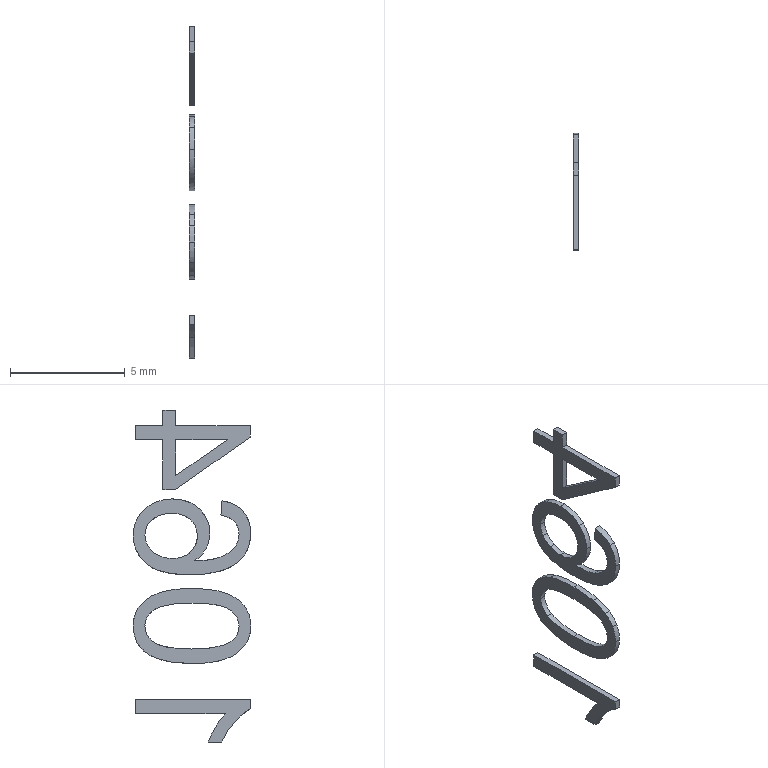Part | STEP file | BBS-JK-ZYBL-1064-H5-1.stp.STEP | 4 solids | 79 faces | box 0.25 x 5.106 x 14.441 mm | volume 6.175 mm3 | spline 51 | plane 28